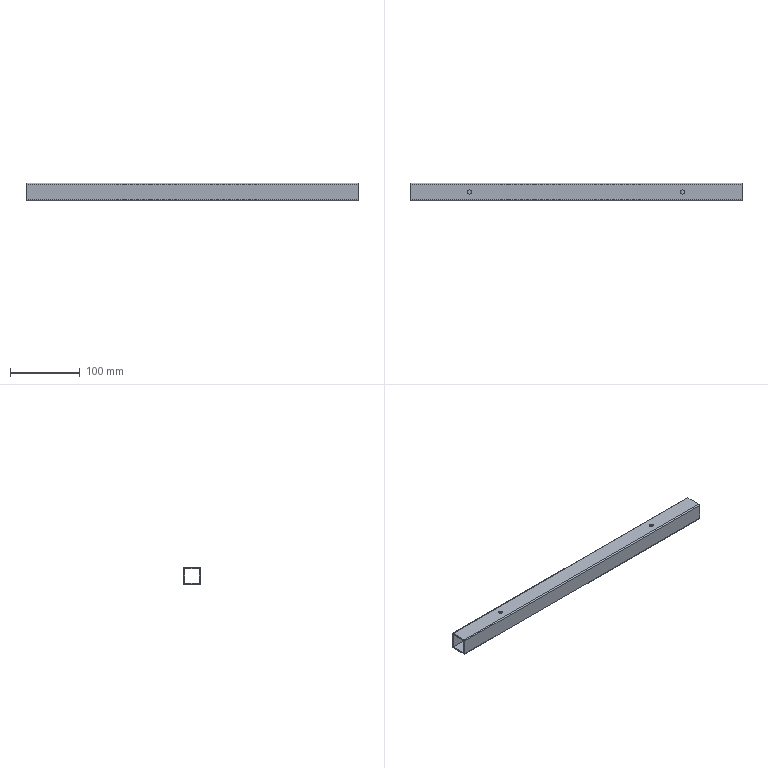Part | NX | features BREP 1 | 1 solid | 18 faces | box 474.98 x 25.4 x 25.4 mm | volume 87017 mm3 | plane 10 | cylinder 8 | commonest cylinder face diameters 3.175 x4 5.842 x4
STEP:
#1=CARTESIAN_POINT('',(-237.49,12.7,-11.113));
#2=VERTEX_POINT('',#1);
#3=CARTESIAN_POINT('',(-237.49,12.7,11.113));
#4=VERTEX_POINT('',#3);
#5=CARTESIAN_POINT('',(-237.49,12.7,-11.113));
#6=DIRECTION('',(0.,0.,1.));
#7=VECTOR('',#6,1000.);
#8=LINE('',#5,#7);
#9=EDGE_CURVE('',#2,#4,#8,.T.);
#10=ORIENTED_EDGE('',*,*,#9,.F.);
#11=CARTESIAN_POINT('',(-237.49,11.113,-12.7));
#12=VERTEX_POINT('',#11);
#13=CARTESIAN_POINT('',(-237.49,11.113,-11.113));
#14=DIRECTION('',(-1.,0.,0.));
#15=DIRECTION('',(0.,1.,0.));
#16=AXIS2_PLACEMENT_3D('',#13,#14,#15);
#17=CIRCLE('',#16,1.587);
#18=EDGE_CURVE('',#2,#12,#17,.T.);
#19=ORIENTED_EDGE('',*,*,#18,.T.);
#20=CARTESIAN_POINT('',(-237.49,-11.113,-12.7));
#21=VERTEX_POINT('',#20);
#22=CARTESIAN_POINT('',(-237.49,-11.113,-12.7));
#23=DIRECTION('',(0.,1.,0.));
#24=VECTOR('',#23,1000.);
#25=LINE('',#22,#24);
#26=EDGE_CURVE('',#21,#12,#25,.T.);
#27=ORIENTED_EDGE('',*,*,#26,.F.);
#28=CARTESIAN_POINT('',(-237.49,-12.7,-11.113));
#29=VERTEX_POINT('',#28);
#30=CARTESIAN_POINT('',(-237.49,-11.113,-11.113));
#31=DIRECTION('',(-1.,0.,0.));
#32=DIRECTION('',(0.,0.,-1.));
#33=AXIS2_PLACEMENT_3D('',#30,#31,#32);
#34=CIRCLE('',#33,1.587);
#35=EDGE_CURVE('',#21,#29,#34,.T.);
#36=ORIENTED_EDGE('',*,*,#35,.T.);
#37=CARTESIAN_POINT('',(-237.49,-12.7,11.113));
#38=VERTEX_POINT('',#37);
#39=CARTESIAN_POINT('',(-237.49,-12.7,11.113));
#40=DIRECTION('',(0.,0.,-1.));
#41=VECTOR('',#40,1000.);
#42=LINE('',#39,#41);
#43=EDGE_CURVE('',#38,#29,#42,.T.);
#44=ORIENTED_EDGE('',*,*,#43,.F.);
#45=CARTESIAN_POINT('',(-237.49,-11.113,12.7));
#46=VERTEX_POINT('',#45);
#47=CARTESIAN_POINT('',(-237.49,-11.113,11.113));
#48=DIRECTION('',(-1.,0.,0.));
#49=DIRECTION('',(0.,-1.,0.));
#50=AXIS2_PLACEMENT_3D('',#47,#48,#49);
#51=CIRCLE('',#50,1.587);
#52=EDGE_CURVE('',#38,#46,#51,.T.);
#53=ORIENTED_EDGE('',*,*,#52,.T.);
#54=CARTESIAN_POINT('',(-237.49,11.113,12.7));
#55=VERTEX_POINT('',#54);
#56=CARTESIAN_POINT('',(-237.49,11.113,12.7));
#57=DIRECTION('',(0.,-1.,0.));
#58=VECTOR('',#57,1000.);
#59=LINE('',#56,#58);
#60=EDGE_CURVE('',#55,#46,#59,.T.);
#61=ORIENTED_EDGE('',*,*,#60,.F.);
#62=CARTESIAN_POINT('',(-237.49,11.113,11.113));
#63=DIRECTION('',(-1.,0.,0.));
#64=DIRECTION('',(0.,0.,1.));
#65=AXIS2_PLACEMENT_3D('',#62,#63,#64);
#66=CIRCLE('',#65,1.587);
#67=EDGE_CURVE('',#55,#4,#66,.T.);
#68=ORIENTED_EDGE('',*,*,#67,.T.);
#69=EDGE_LOOP('',(#10,#19,#27,#36,#44,#53,#61,#68));
#70=FACE_BOUND('',#69,.T.);
#71=CARTESIAN_POINT('',(-237.49,10.719,10.719));
#72=VERTEX_POINT('',#71);
#73=CARTESIAN_POINT('',(-237.49,10.719,-10.719));
#74=VERTEX_POINT('',#73);
#75=CARTESIAN_POINT('',(-237.49,10.719,10.719));
#76=DIRECTION('',(0.,0.,-1.));
#77=VECTOR('',#76,1000.);
#78=LINE('',#75,#77);
#79=EDGE_CURVE('',#72,#74,#78,.T.);
#80=ORIENTED_EDGE('',*,*,#79,.F.);
#81=CARTESIAN_POINT('',(-237.49,-10.719,10.719));
#82=VERTEX_POINT('',#81);
#83=CARTESIAN_POINT('',(-237.49,-10.719,10.719));
#84=DIRECTION('',(0.,1.,0.));
#85=VECTOR('',#84,1000.);
#86=LINE('',#83,#85);
#87=EDGE_CURVE('',#82,#72,#86,.T.);
#88=ORIENTED_EDGE('',*,*,#87,.F.);
#89=CARTESIAN_POINT('',(-237.49,-10.719,-10.719));
#90=VERTEX_POINT('',#89);
#91=CARTESIAN_POINT('',(-237.49,-10.719,-10.719));
#92=DIRECTION('',(0.,0.,1.));
#93=VECTOR('',#92,1000.);
#94=LINE('',#91,#93);
#95=EDGE_CURVE('',#90,#82,#94,.T.);
#96=ORIENTED_EDGE('',*,*,#95,.F.);
#97=CARTESIAN_POINT('',(-237.49,10.719,-10.719));
#98=DIRECTION('',(0.,-1.,0.));
#99=VECTOR('',#98,1000.);
#100=LINE('',#97,#99);
#101=EDGE_CURVE('',#74,#90,#100,.T.);
#102=ORIENTED_EDGE('',*,*,#101,.F.);
#103=EDGE_LOOP('',(#80,#88,#96,#102));
#104=FACE_BOUND('',#103,.T.);
#105=CARTESIAN_POINT('',(-237.49,0.,0.));
#106=DIRECTION('',(1.,0.,0.));
#107=DIRECTION('',(0.,1.,0.));
#108=AXIS2_PLACEMENT_3D('',#105,#106,#107);
#109=PLANE('',#108);
#110=ADVANCED_FACE('',(#70,#104),#109,.F.);
#111=CARTESIAN_POINT('',(237.49,-10.719,-10.719));
#112=VERTEX_POINT('',#111);
#113=CARTESIAN_POINT('',(-237.49,-10.719,-10.719));
#114=DIRECTION('',(1.,0.,0.));
#115=VECTOR('',#114,1000.);
#116=LINE('',#113,#115);
#117=EDGE_CURVE('',#90,#112,#116,.T.);
#118=ORIENTED_EDGE('',*,*,#117,.T.);
#119=CARTESIAN_POINT('',(237.49,10.719,-10.719));
#120=VERTEX_POINT('',#119);
#121=CARTESIAN_POINT('',(237.49,10.719,-10.719));
#122=DIRECTION('',(0.,-1.,0.));
#123=VECTOR('',#122,1000.);
#124=LINE('',#121,#123);
#125=EDGE_CURVE('',#120,#112,#124,.T.);
#126=ORIENTED_EDGE('',*,*,#125,.F.);
#127=CARTESIAN_POINT('',(-237.49,10.719,-10.719));
#128=DIRECTION('',(1.,0.,0.));
#129=VECTOR('',#128,1000.);
#130=LINE('',#127,#129);
#131=EDGE_CURVE('',#74,#120,#130,.T.);
#132=ORIENTED_EDGE('',*,*,#131,.F.);
#133=ORIENTED_EDGE('',*,*,#101,.T.);
#134=EDGE_LOOP('',(#118,#126,#132,#133));
#135=FACE_BOUND('',#134,.T.);
#136=CARTESIAN_POINT('',(-237.49,10.719,-10.719));
#137=DIRECTION('',(0.,0.,1.));
#138=DIRECTION('',(1.,0.,0.));
#139=AXIS2_PLACEMENT_3D('',#136,#137,#138);
#140=PLANE('',#139);
#141=ADVANCED_FACE('',(#135),#140,.T.);
#142=ORIENTED_EDGE('',*,*,#131,.T.);
#143=CARTESIAN_POINT('',(237.49,10.719,10.719));
#144=VERTEX_POINT('',#143);
#145=CARTESIAN_POINT('',(237.49,10.719,10.719));
#146=DIRECTION('',(0.,0.,-1.));
#147=VECTOR('',#146,1000.);
#148=LINE('',#145,#147);
#149=EDGE_CURVE('',#144,#120,#148,.T.);
#150=ORIENTED_EDGE('',*,*,#149,.F.);
#151=CARTESIAN_POINT('',(-237.49,10.719,10.719));
#152=DIRECTION('',(1.,0.,0.));
#153=VECTOR('',#152,1000.);
#154=LINE('',#151,#153);
#155=EDGE_CURVE('',#72,#144,#154,.T.);
#156=ORIENTED_EDGE('',*,*,#155,.F.);
#157=ORIENTED_EDGE('',*,*,#79,.T.);
#158=EDGE_LOOP('',(#142,#150,#156,#157));
#159=FACE_BOUND('',#158,.T.);
#160=CARTESIAN_POINT('',(-237.49,10.719,10.719));
#161=DIRECTION('',(0.,-1.,0.));
#162=DIRECTION('',(0.,0.,-1.));
#163=AXIS2_PLACEMENT_3D('',#160,#161,#162);
#164=PLANE('',#163);
#165=ADVANCED_FACE('',(#159),#164,.T.);
#166=ORIENTED_EDGE('',*,*,#155,.T.);
#167=CARTESIAN_POINT('',(237.49,-10.719,10.719));
#168=VERTEX_POINT('',#167);
#169=CARTESIAN_POINT('',(237.49,-10.719,10.719));
#170=DIRECTION('',(0.,1.,0.));
#171=VECTOR('',#170,1000.);
#172=LINE('',#169,#171);
#173=EDGE_CURVE('',#168,#144,#172,.T.);
#174=ORIENTED_EDGE('',*,*,#173,.F.);
#175=CARTESIAN_POINT('',(-237.49,-10.719,10.719));
#176=DIRECTION('',(1.,0.,0.));
#177=VECTOR('',#176,1000.);
#178=LINE('',#175,#177);
#179=EDGE_CURVE('',#82,#168,#178,.T.);
#180=ORIENTED_EDGE('',*,*,#179,.F.);
#181=ORIENTED_EDGE('',*,*,#87,.T.);
#182=EDGE_LOOP('',(#166,#174,#180,#181));
#183=FACE_BOUND('',#182,.T.);
#184=CARTESIAN_POINT('',(149.479,0.,10.719));
#185=VERTEX_POINT('',#184);
#186=CARTESIAN_POINT('',(155.321,0.,10.719));
#187=VERTEX_POINT('',#186);
#188=CARTESIAN_POINT('',(152.4,0.,10.719));
#189=DIRECTION('',(0.,0.,1.));
#190=DIRECTION('',(-1.,0.,0.));
#191=AXIS2_PLACEMENT_3D('',#188,#189,#190);
#192=CIRCLE('',#191,2.921);
#193=EDGE_CURVE('',#185,#187,#192,.T.);
#194=ORIENTED_EDGE('',*,*,#193,.T.);
#195=CARTESIAN_POINT('',(152.4,0.,10.719));
#196=DIRECTION('',(0.,0.,1.));
#197=DIRECTION('',(1.,0.,0.));
#198=AXIS2_PLACEMENT_3D('',#195,#196,#197);
#199=CIRCLE('',#198,2.921);
#200=EDGE_CURVE('',#187,#185,#199,.T.);
#201=ORIENTED_EDGE('',*,*,#200,.T.);
#202=EDGE_LOOP('',(#194,#201));
#203=FACE_BOUND('',#202,.T.);
#204=CARTESIAN_POINT('',(-155.321,0.,10.719));
#205=VERTEX_POINT('',#204);
#206=CARTESIAN_POINT('',(-149.479,0.,10.719));
#207=VERTEX_POINT('',#206);
#208=CARTESIAN_POINT('',(-152.4,0.,10.719));
#209=DIRECTION('',(0.,0.,1.));
#210=DIRECTION('',(-1.,0.,0.));
#211=AXIS2_PLACEMENT_3D('',#208,#209,#210);
#212=CIRCLE('',#211,2.921);
#213=EDGE_CURVE('',#205,#207,#212,.T.);
#214=ORIENTED_EDGE('',*,*,#213,.T.);
#215=CARTESIAN_POINT('',(-152.4,0.,10.719));
#216=DIRECTION('',(0.,0.,1.));
#217=DIRECTION('',(1.,0.,0.));
#218=AXIS2_PLACEMENT_3D('',#215,#216,#217);
#219=CIRCLE('',#218,2.921);
#220=EDGE_CURVE('',#207,#205,#219,.T.);
#221=ORIENTED_EDGE('',*,*,#220,.T.);
#222=EDGE_LOOP('',(#214,#221));
#223=FACE_BOUND('',#222,.T.);
#224=CARTESIAN_POINT('',(-237.49,-10.719,10.719));
#225=DIRECTION('',(0.,0.,-1.));
#226=DIRECTION('',(0.,-1.,0.));
#227=AXIS2_PLACEMENT_3D('',#224,#225,#226);
#228=PLANE('',#227);
#229=ADVANCED_FACE('',(#183,#203,#223),#228,.T.);
#230=ORIENTED_EDGE('',*,*,#179,.T.);
#231=CARTESIAN_POINT('',(237.49,-10.719,-10.719));
#232=DIRECTION('',(0.,0.,1.));
#233=VECTOR('',#232,1000.);
#234=LINE('',#231,#233);
#235=EDGE_CURVE('',#112,#168,#234,.T.);
#236=ORIENTED_EDGE('',*,*,#235,.F.);
#237=ORIENTED_EDGE('',*,*,#117,.F.);
#238=ORIENTED_EDGE('',*,*,#95,.T.);
#239=EDGE_LOOP('',(#230,#236,#237,#238));
#240=FACE_BOUND('',#239,.T.);
#241=CARTESIAN_POINT('',(-237.49,-10.719,-10.719));
#242=DIRECTION('',(0.,1.,0.));
#243=DIRECTION('',(1.,0.,0.));
#244=AXIS2_PLACEMENT_3D('',#241,#242,#243);
#245=PLANE('',#244);
#246=ADVANCED_FACE('',(#240),#245,.T.);
#247=CARTESIAN_POINT('',(237.49,11.113,12.7));
#248=VERTEX_POINT('',#247);
#249=CARTESIAN_POINT('',(237.49,-11.113,12.7));
#250=VERTEX_POINT('',#249);
#251=CARTESIAN_POINT('',(237.49,11.113,12.7));
#252=DIRECTION('',(0.,-1.,0.));
#253=VECTOR('',#252,1000.);
#254=LINE('',#251,#253);
#255=EDGE_CURVE('',#248,#250,#254,.T.);
#256=ORIENTED_EDGE('',*,*,#255,.T.);
#257=CARTESIAN_POINT('',(237.49,-12.7,11.113));
#258=VERTEX_POINT('',#257);
#259=CARTESIAN_POINT('',(237.49,-11.113,11.113));
#260=DIRECTION('',(1.,0.,0.));
#261=DIRECTION('',(0.,0.,1.));
#262=AXIS2_PLACEMENT_3D('',#259,#260,#261);
#263=CIRCLE('',#262,1.587);
#264=EDGE_CURVE('',#250,#258,#263,.T.);
#265=ORIENTED_EDGE('',*,*,#264,.T.);
#266=CARTESIAN_POINT('',(237.49,-12.7,-11.113));
#267=VERTEX_POINT('',#266);
#268=CARTESIAN_POINT('',(237.49,-12.7,11.113));
#269=DIRECTION('',(0.,0.,-1.));
#270=VECTOR('',#269,1000.);
#271=LINE('',#268,#270);
#272=EDGE_CURVE('',#258,#267,#271,.T.);
#273=ORIENTED_EDGE('',*,*,#272,.T.);
#274=CARTESIAN_POINT('',(237.49,-11.113,-12.7));
#275=VERTEX_POINT('',#274);
#276=CARTESIAN_POINT('',(237.49,-11.113,-11.113));
#277=DIRECTION('',(1.,0.,0.));
#278=DIRECTION('',(0.,-1.,0.));
#279=AXIS2_PLACEMENT_3D('',#276,#277,#278);
#280=CIRCLE('',#279,1.587);
#281=EDGE_CURVE('',#267,#275,#280,.T.);
#282=ORIENTED_EDGE('',*,*,#281,.T.);
#283=CARTESIAN_POINT('',(237.49,11.113,-12.7));
#284=VERTEX_POINT('',#283);
#285=CARTESIAN_POINT('',(237.49,-11.113,-12.7));
#286=DIRECTION('',(0.,1.,0.));
#287=VECTOR('',#286,1000.);
#288=LINE('',#285,#287);
#289=EDGE_CURVE('',#275,#284,#288,.T.);
#290=ORIENTED_EDGE('',*,*,#289,.T.);
#291=CARTESIAN_POINT('',(237.49,12.7,-11.113));
#292=VERTEX_POINT('',#291);
#293=CARTESIAN_POINT('',(237.49,11.113,-11.113));
#294=DIRECTION('',(1.,0.,0.));
#295=DIRECTION('',(0.,0.,-1.));
#296=AXIS2_PLACEMENT_3D('',#293,#294,#295);
#297=CIRCLE('',#296,1.587);
#298=EDGE_CURVE('',#284,#292,#297,.T.);
#299=ORIENTED_EDGE('',*,*,#298,.T.);
#300=CARTESIAN_POINT('',(237.49,12.7,11.113));
#301=VERTEX_POINT('',#300);
#302=CARTESIAN_POINT('',(237.49,12.7,-11.113));
#303=DIRECTION('',(0.,0.,1.));
#304=VECTOR('',#303,1000.);
#305=LINE('',#302,#304);
#306=EDGE_CURVE('',#292,#301,#305,.T.);
#307=ORIENTED_EDGE('',*,*,#306,.T.);
#308=CARTESIAN_POINT('',(237.49,11.113,11.113));
#309=DIRECTION('',(1.,0.,0.));
#310=DIRECTION('',(0.,1.,0.));
#311=AXIS2_PLACEMENT_3D('',#308,#309,#310);
#312=CIRCLE('',#311,1.587);
#313=EDGE_CURVE('',#301,#248,#312,.T.);
#314=ORIENTED_EDGE('',*,*,#313,.T.);
#315=EDGE_LOOP('',(#256,#265,#273,#282,#290,#299,#307,#314));
#316=FACE_BOUND('',#315,.T.);
#317=ORIENTED_EDGE('',*,*,#235,.T.);
#318=ORIENTED_EDGE('',*,*,#173,.T.);
#319=ORIENTED_EDGE('',*,*,#149,.T.);
#320=ORIENTED_EDGE('',*,*,#125,.T.);
#321=EDGE_LOOP('',(#317,#318,#319,#320));
#322=FACE_BOUND('',#321,.T.);
#323=CARTESIAN_POINT('',(237.49,0.,0.));
#324=DIRECTION('',(1.,0.,0.));
#325=DIRECTION('',(0.,1.,0.));
#326=AXIS2_PLACEMENT_3D('',#323,#324,#325);
#327=PLANE('',#326);
#328=ADVANCED_FACE('',(#316,#322),#327,.T.);
#329=ORIENTED_EDGE('',*,*,#313,.F.);
#330=CARTESIAN_POINT('',(237.49,12.7,11.113));
#331=DIRECTION('',(-1.,0.,0.));
#332=VECTOR('',#331,1000.);
#333=LINE('',#330,#332);
#334=EDGE_CURVE('',#301,#4,#333,.T.);
#335=ORIENTED_EDGE('',*,*,#334,.T.);
#336=ORIENTED_EDGE('',*,*,#67,.F.);
#337=CARTESIAN_POINT('',(237.49,11.113,12.7));
#338=DIRECTION('',(-1.,0.,0.));
#339=VECTOR('',#338,1000.);
#340=LINE('',#337,#339);
#341=EDGE_CURVE('',#248,#55,#340,.T.);
#342=ORIENTED_EDGE('',*,*,#341,.F.);
#343=EDGE_LOOP('',(#329,#335,#336,#342));
#344=FACE_BOUND('',#343,.T.);
#345=CARTESIAN_POINT('',(238.235,11.113,11.113));
#346=DIRECTION('',(-1.,0.,0.));
#347=DIRECTION('',(0.,0.,1.));
#348=AXIS2_PLACEMENT_3D('',#345,#346,#347);
#349=CYLINDRICAL_SURFACE('',#348,1.587);
#350=ADVANCED_FACE('',(#344),#349,.T.);
#351=ORIENTED_EDGE('',*,*,#60,.T.);
#352=CARTESIAN_POINT('',(237.49,-11.113,12.7));
#353=DIRECTION('',(-1.,0.,0.));
#354=VECTOR('',#353,1000.);
#355=LINE('',#352,#354);
#356=EDGE_CURVE('',#250,#46,#355,.T.);
#357=ORIENTED_EDGE('',*,*,#356,.F.);
#358=ORIENTED_EDGE('',*,*,#255,.F.);
#359=ORIENTED_EDGE('',*,*,#341,.T.);
#360=EDGE_LOOP('',(#351,#357,#358,#359));
#361=FACE_BOUND('',#360,.T.);
#362=CARTESIAN_POINT('',(149.479,0.,12.7));
#363=VERTEX_POINT('',#362);
#364=CARTESIAN_POINT('',(155.321,0.,12.7));
#365=VERTEX_POINT('',#364);
#366=CARTESIAN_POINT('',(152.4,0.,12.7));
#367=DIRECTION('',(0.,0.,1.));
#368=DIRECTION('',(-1.,0.,0.));
#369=AXIS2_PLACEMENT_3D('',#366,#367,#368);
#370=CIRCLE('',#369,2.921);
#371=EDGE_CURVE('',#363,#365,#370,.T.);
#372=ORIENTED_EDGE('',*,*,#371,.F.);
#373=CARTESIAN_POINT('',(152.4,0.,12.7));
#374=DIRECTION('',(0.,0.,1.));
#375=DIRECTION('',(1.,0.,0.));
#376=AXIS2_PLACEMENT_3D('',#373,#374,#375);
#377=CIRCLE('',#376,2.921);
#378=EDGE_CURVE('',#365,#363,#377,.T.);
#379=ORIENTED_EDGE('',*,*,#378,.F.);
#380=EDGE_LOOP('',(#372,#379));
#381=FACE_BOUND('',#380,.T.);
#382=CARTESIAN_POINT('',(-155.321,0.,12.7));
#383=VERTEX_POINT('',#382);
#384=CARTESIAN_POINT('',(-149.479,0.,12.7));
#385=VERTEX_POINT('',#384);
#386=CARTESIAN_POINT('',(-152.4,0.,12.7));
#387=DIRECTION('',(0.,0.,1.));
#388=DIRECTION('',(-1.,0.,0.));
#389=AXIS2_PLACEMENT_3D('',#386,#387,#388);
#390=CIRCLE('',#389,2.921);
#391=EDGE_CURVE('',#383,#385,#390,.T.);
#392=ORIENTED_EDGE('',*,*,#391,.F.);
#393=CARTESIAN_POINT('',(-152.4,0.,12.7));
#394=DIRECTION('',(0.,0.,1.));
#395=DIRECTION('',(1.,0.,0.));
#396=AXIS2_PLACEMENT_3D('',#393,#394,#395);
#397=CIRCLE('',#396,2.921);
#398=EDGE_CURVE('',#385,#383,#397,.T.);
#399=ORIENTED_EDGE('',*,*,#398,.F.);
#400=EDGE_LOOP('',(#392,#399));
#401=FACE_BOUND('',#400,.T.);
#402=CARTESIAN_POINT('',(-237.49,12.7,12.7));
#403=DIRECTION('',(0.,0.,1.));
#404=DIRECTION('',(1.,0.,0.));
#405=AXIS2_PLACEMENT_3D('',#402,#403,#404);
#406=PLANE('',#405);
#407=ADVANCED_FACE('',(#361,#381,#401),#406,.T.);
#408=ORIENTED_EDGE('',*,*,#264,.F.);
#409=ORIENTED_EDGE('',*,*,#356,.T.);
#410=ORIENTED_EDGE('',*,*,#52,.F.);
#411=CARTESIAN_POINT('',(237.49,-12.7,11.113));
#412=DIRECTION('',(-1.,0.,0.));
#413=VECTOR('',#412,1000.);
#414=LINE('',#411,#413);
#415=EDGE_CURVE('',#258,#38,#414,.T.);
#416=ORIENTED_EDGE('',*,*,#415,.F.);
#417=EDGE_LOOP('',(#408,#409,#410,#416));
#418=FACE_BOUND('',#417,.T.);
#419=CARTESIAN_POINT('',(238.235,-11.113,11.113));
#420=DIRECTION('',(-1.,0.,0.));
#421=DIRECTION('',(0.,-1.,0.));
#422=AXIS2_PLACEMENT_3D('',#419,#420,#421);
#423=CYLINDRICAL_SURFACE('',#422,1.587);
#424=ADVANCED_FACE('',(#418),#423,.T.);
#425=ORIENTED_EDGE('',*,*,#43,.T.);
#426=CARTESIAN_POINT('',(237.49,-12.7,-11.113));
#427=DIRECTION('',(-1.,0.,0.));
#428=VECTOR('',#427,1000.);
#429=LINE('',#426,#428);
#430=EDGE_CURVE('',#267,#29,#429,.T.);
#431=ORIENTED_EDGE('',*,*,#430,.F.);
#432=ORIENTED_EDGE('',*,*,#272,.F.);
#433=ORIENTED_EDGE('',*,*,#415,.T.);
#434=EDGE_LOOP('',(#425,#431,#432,#433));
#435=FACE_BOUND('',#434,.T.);
#436=CARTESIAN_POINT('',(-237.49,-12.7,12.7));
#437=DIRECTION('',(0.,-1.,0.));
#438=DIRECTION('',(0.,0.,-1.));
#439=AXIS2_PLACEMENT_3D('',#436,#437,#438);
#440=PLANE('',#439);
#441=ADVANCED_FACE('',(#435),#440,.T.);
#442=ORIENTED_EDGE('',*,*,#281,.F.);
#443=ORIENTED_EDGE('',*,*,#430,.T.);
#444=ORIENTED_EDGE('',*,*,#35,.F.);
#445=CARTESIAN_POINT('',(237.49,-11.113,-12.7));
#446=DIRECTION('',(-1.,0.,0.));
#447=VECTOR('',#446,1000.);
#448=LINE('',#445,#447);
#449=EDGE_CURVE('',#275,#21,#448,.T.);
#450=ORIENTED_EDGE('',*,*,#449,.F.);
#451=EDGE_LOOP('',(#442,#443,#444,#450));
#452=FACE_BOUND('',#451,.T.);
#453=CARTESIAN_POINT('',(238.235,-11.113,-11.113));
#454=DIRECTION('',(-1.,0.,0.));
#455=DIRECTION('',(0.,0.,-1.));
#456=AXIS2_PLACEMENT_3D('',#453,#454,#455);
#457=CYLINDRICAL_SURFACE('',#456,1.587);
#458=ADVANCED_FACE('',(#452),#457,.T.);
#459=ORIENTED_EDGE('',*,*,#289,.F.);
#460=ORIENTED_EDGE('',*,*,#449,.T.);
#461=ORIENTED_EDGE('',*,*,#26,.T.);
#462=CARTESIAN_POINT('',(237.49,11.113,-12.7));
#463=DIRECTION('',(-1.,0.,0.));
#464=VECTOR('',#463,1000.);
#465=LINE('',#462,#464);
#466=EDGE_CURVE('',#284,#12,#465,.T.);
#467=ORIENTED_EDGE('',*,*,#466,.F.);
#468=EDGE_LOOP('',(#459,#460,#461,#467));
#469=FACE_BOUND('',#468,.T.);
#470=CARTESIAN_POINT('',(-237.49,-12.7,-12.7));
#471=DIRECTION('',(0.,0.,-1.));
#472=DIRECTION('',(0.,-1.,0.));
#473=AXIS2_PLACEMENT_3D('',#470,#471,#472);
#474=PLANE('',#473);
#475=ADVANCED_FACE('',(#469),#474,.T.);
#476=ORIENTED_EDGE('',*,*,#298,.F.);
#477=ORIENTED_EDGE('',*,*,#466,.T.);
#478=ORIENTED_EDGE('',*,*,#18,.F.);
#479=CARTESIAN_POINT('',(237.49,12.7,-11.113));
#480=DIRECTION('',(-1.,0.,0.));
#481=VECTOR('',#480,1000.);
#482=LINE('',#479,#481);
#483=EDGE_CURVE('',#292,#2,#482,.T.);
#484=ORIENTED_EDGE('',*,*,#483,.F.);
#485=EDGE_LOOP('',(#476,#477,#478,#484));
#486=FACE_BOUND('',#485,.T.);
#487=CARTESIAN_POINT('',(238.235,11.113,-11.113));
#488=DIRECTION('',(-1.,0.,0.));
#489=DIRECTION('',(0.,1.,0.));
#490=AXIS2_PLACEMENT_3D('',#487,#488,#489);
#491=CYLINDRICAL_SURFACE('',#490,1.587);
#492=ADVANCED_FACE('',(#486),#491,.T.);
#493=ORIENTED_EDGE('',*,*,#306,.F.);
#494=ORIENTED_EDGE('',*,*,#483,.T.);
#495=ORIENTED_EDGE('',*,*,#9,.T.);
#496=ORIENTED_EDGE('',*,*,#334,.F.);
#497=EDGE_LOOP('',(#493,#494,#495,#496));
#498=FACE_BOUND('',#497,.T.);
#499=CARTESIAN_POINT('',(-237.49,12.7,-12.7));
#500=DIRECTION('',(0.,1.,0.));
#501=DIRECTION('',(1.,0.,0.));
#502=AXIS2_PLACEMENT_3D('',#499,#500,#501);
#503=PLANE('',#502);
#504=ADVANCED_FACE('',(#498),#503,.T.);
#505=CARTESIAN_POINT('',(149.479,0.,12.7));
#506=DIRECTION('',(0.,0.,-1.));
#507=VECTOR('',#506,1000.);
#508=LINE('',#505,#507);
#509=EDGE_CURVE('',#363,#185,#508,.T.);
#510=ORIENTED_EDGE('',*,*,#509,.T.);
#511=ORIENTED_EDGE('',*,*,#200,.F.);
#512=CARTESIAN_POINT('',(155.321,0.,12.7));
#513=DIRECTION('',(0.,0.,-1.));
#514=VECTOR('',#513,1000.);
#515=LINE('',#512,#514);
#516=EDGE_CURVE('',#365,#187,#515,.T.);
#517=ORIENTED_EDGE('',*,*,#516,.F.);
#518=ORIENTED_EDGE('',*,*,#378,.T.);
#519=EDGE_LOOP('',(#510,#511,#517,#518));
#520=FACE_BOUND('',#519,.T.);
#521=CARTESIAN_POINT('',(152.4,0.,12.7));
#522=DIRECTION('',(0.,0.,1.));
#523=DIRECTION('',(1.,0.,0.));
#524=AXIS2_PLACEMENT_3D('',#521,#522,#523);
#525=CYLINDRICAL_SURFACE('',#524,2.921);
#526=ADVANCED_FACE('',(#520),#525,.F.);
#527=ORIENTED_EDGE('',*,*,#516,.T.);
#528=ORIENTED_EDGE('',*,*,#193,.F.);
#529=ORIENTED_EDGE('',*,*,#509,.F.);
#530=ORIENTED_EDGE('',*,*,#371,.T.);
#531=EDGE_LOOP('',(#527,#528,#529,#530));
#532=FACE_BOUND('',#531,.T.);
#533=CARTESIAN_POINT('',(152.4,0.,12.7));
#534=DIRECTION('',(0.,0.,1.));
#535=DIRECTION('',(1.,0.,0.));
#536=AXIS2_PLACEMENT_3D('',#533,#534,#535);
#537=CYLINDRICAL_SURFACE('',#536,2.921);
#538=ADVANCED_FACE('',(#532),#537,.F.);
#539=CARTESIAN_POINT('',(-155.321,0.,12.7));
#540=DIRECTION('',(0.,0.,-1.));
#541=VECTOR('',#540,1000.);
#542=LINE('',#539,#541);
#543=EDGE_CURVE('',#383,#205,#542,.T.);
#544=ORIENTED_EDGE('',*,*,#543,.T.);
#545=ORIENTED_EDGE('',*,*,#220,.F.);
#546=CARTESIAN_POINT('',(-149.479,0.,12.7));
#547=DIRECTION('',(0.,0.,-1.));
#548=VECTOR('',#547,1000.);
#549=LINE('',#546,#548);
#550=EDGE_CURVE('',#385,#207,#549,.T.);
#551=ORIENTED_EDGE('',*,*,#550,.F.);
#552=ORIENTED_EDGE('',*,*,#398,.T.);
#553=EDGE_LOOP('',(#544,#545,#551,#552));
#554=FACE_BOUND('',#553,.T.);
#555=CARTESIAN_POINT('',(-152.4,0.,12.7));
#556=DIRECTION('',(0.,0.,1.));
#557=DIRECTION('',(1.,0.,0.));
#558=AXIS2_PLACEMENT_3D('',#555,#556,#557);
#559=CYLINDRICAL_SURFACE('',#558,2.921);
#560=ADVANCED_FACE('',(#554),#559,.F.);
#561=ORIENTED_EDGE('',*,*,#550,.T.);
#562=ORIENTED_EDGE('',*,*,#213,.F.);
#563=ORIENTED_EDGE('',*,*,#543,.F.);
#564=ORIENTED_EDGE('',*,*,#391,.T.);
#565=EDGE_LOOP('',(#561,#562,#563,#564));
#566=FACE_BOUND('',#565,.T.);
#567=CARTESIAN_POINT('',(-152.4,0.,12.7));
#568=DIRECTION('',(0.,0.,1.));
#569=DIRECTION('',(1.,0.,0.));
#570=AXIS2_PLACEMENT_3D('',#567,#568,#569);
#571=CYLINDRICAL_SURFACE('',#570,2.921);
#572=ADVANCED_FACE('',(#566),#571,.F.);
#573=CLOSED_SHELL('',(#110,#141,#165,#229,#246,#328,#350,#407,#424,#441,#458,#475,#492,#504,#526,#538,#560,#572));
#574=MANIFOLD_SOLID_BREP('',#573);
#575=(LENGTH_UNIT()NAMED_UNIT(*)SI_UNIT(.MILLI.,.METRE.));
#576=UNCERTAINTY_MEASURE_WITH_UNIT(LENGTH_MEASURE(0.00001),#575,'','');
#577=(NAMED_UNIT(*)PLANE_ANGLE_UNIT()SI_UNIT($,.RADIAN.));
#578=(NAMED_UNIT(*)SI_UNIT($,.STERADIAN.)SOLID_ANGLE_UNIT());
#579=(GEOMETRIC_REPRESENTATION_CONTEXT(3)GLOBAL_UNCERTAINTY_ASSIGNED_CONTEXT((#576))GLOBAL_UNIT_ASSIGNED_CONTEXT((#575,#577,#578))REPRESENTATION_CONTEXT('',''));
#580=ADVANCED_BREP_SHAPE_REPRESENTATION('',(#574),#579);